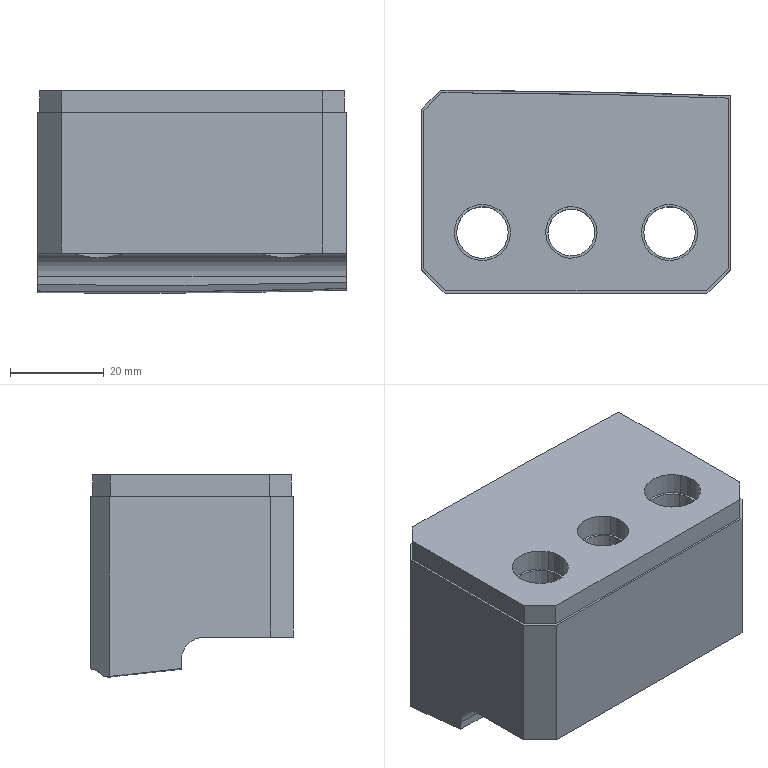Part | CATIA | 2 solids | 45 faces | box 66 x 43.369 x 43.322 mm | volume 92205 mm3 | plane 20 | cylinder 17 | spline 5 | other 3 | commonest cylinder face diameters 11 x6 12 x4 18 x4 10 x3